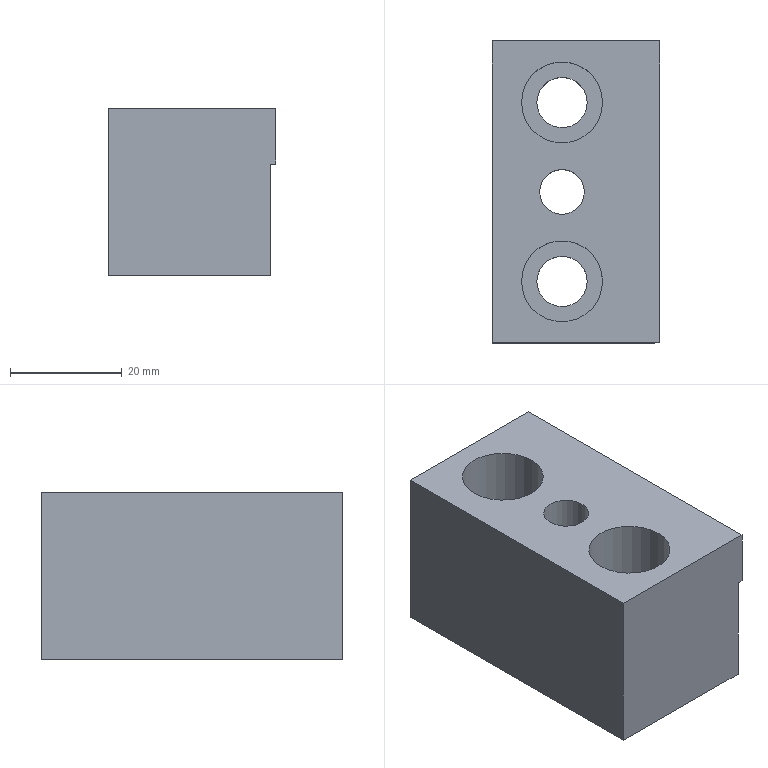Part | NX | features 23 2 | 1 solid | 15 faces | box 30 x 54 x 30 mm | volume 39961 mm3 | plane 10 | cylinder 5 | commonest cylinder face diameters 9 x2 14.5 x2 8.001 x1
STEP:
#1=CARTESIAN_POINT('',(3684.199,-436.,-14.5));
#2=VERTEX_POINT('',#1);
#3=CARTESIAN_POINT('',(3688.699,-436.,-14.5));
#4=DIRECTION('',(0.,0.,-1.));
#5=DIRECTION('',(-1.,0.,0.));
#6=AXIS2_PLACEMENT_3D('',#3,#4,#5);
#7=CIRCLE('',#6,4.5);
#8=EDGE_CURVE('',#2,#2,#7,.T.);
#9=ORIENTED_EDGE('',*,*,#8,.T.);
#10=EDGE_LOOP('',(#9));
#11=FACE_BOUND('',#10,.T.);
#12=CARTESIAN_POINT('',(3681.449,-436.,-14.5));
#13=VERTEX_POINT('',#12);
#14=CARTESIAN_POINT('',(3688.699,-436.,-14.5));
#15=DIRECTION('',(0.,0.,-1.));
#16=DIRECTION('',(-1.,0.,0.));
#17=AXIS2_PLACEMENT_3D('',#14,#15,#16);
#18=CIRCLE('',#17,7.25);
#19=EDGE_CURVE('',#13,#13,#18,.T.);
#20=ORIENTED_EDGE('',*,*,#19,.F.);
#21=EDGE_LOOP('',(#20));
#22=FACE_BOUND('',#21,.T.);
#23=CARTESIAN_POINT('',(3688.699,-436.,-14.5));
#24=DIRECTION('',(0.,0.,-1.));
#25=DIRECTION('',(-1.,0.,0.));
#26=AXIS2_PLACEMENT_3D('',#23,#24,#25);
#27=PLANE('',#26);
#28=ADVANCED_FACE('',(#11,#22),#27,.F.);
#29=CARTESIAN_POINT('',(3705.199,-393.,-13.5));
#30=VERTEX_POINT('',#29);
#31=CARTESIAN_POINT('',(3705.199,-447.,-13.5));
#32=VERTEX_POINT('',#31);
#33=CARTESIAN_POINT('',(3705.199,-407.5,-13.5));
#34=DIRECTION('',(0.,-1.,0.));
#35=VECTOR('',#34,1000.);
#36=LINE('',#33,#35);
#37=EDGE_CURVE('',#30,#32,#36,.T.);
#38=ORIENTED_EDGE('',*,*,#37,.F.);
#39=CARTESIAN_POINT('',(3706.199,-393.,-13.5));
#40=VERTEX_POINT('',#39);
#41=CARTESIAN_POINT('',(3678.699,-393.,-13.5));
#42=DIRECTION('',(-1.,0.,0.));
#43=VECTOR('',#42,1000.);
#44=LINE('',#41,#43);
#45=EDGE_CURVE('',#40,#30,#44,.T.);
#46=ORIENTED_EDGE('',*,*,#45,.F.);
#47=CARTESIAN_POINT('',(3706.199,-447.,-13.5));
#48=VERTEX_POINT('',#47);
#49=CARTESIAN_POINT('',(3706.199,-407.5,-13.5));
#50=DIRECTION('',(0.,1.,0.));
#51=VECTOR('',#50,1000.);
#52=LINE('',#49,#51);
#53=EDGE_CURVE('',#48,#40,#52,.T.);
#54=ORIENTED_EDGE('',*,*,#53,.F.);
#55=CARTESIAN_POINT('',(3706.199,-447.,-13.5));
#56=DIRECTION('',(1.,0.,0.));
#57=VECTOR('',#56,1000.);
#58=LINE('',#55,#57);
#59=EDGE_CURVE('',#32,#48,#58,.T.);
#60=ORIENTED_EDGE('',*,*,#59,.F.);
#61=EDGE_LOOP('',(#38,#46,#54,#60));
#62=FACE_BOUND('',#61,.T.);
#63=CARTESIAN_POINT('',(3691.199,-420.,-13.5));
#64=DIRECTION('',(0.,0.,1.));
#65=DIRECTION('',(1.,0.,0.));
#66=AXIS2_PLACEMENT_3D('',#63,#64,#65);
#67=PLANE('',#66);
#68=ADVANCED_FACE('',(#62),#67,.F.);
#69=ORIENTED_EDGE('',*,*,#8,.F.);
#70=EDGE_LOOP('',(#69));
#71=FACE_BOUND('',#70,.T.);
#72=CARTESIAN_POINT('',(3684.199,-436.,-33.5));
#73=VERTEX_POINT('',#72);
#74=CARTESIAN_POINT('',(3688.699,-436.,-33.5));
#75=DIRECTION('',(0.,0.,1.));
#76=DIRECTION('',(-1.,0.,0.));
#77=AXIS2_PLACEMENT_3D('',#74,#75,#76);
#78=CIRCLE('',#77,4.5);
#79=EDGE_CURVE('',#73,#73,#78,.T.);
#80=ORIENTED_EDGE('',*,*,#79,.F.);
#81=EDGE_LOOP('',(#80));
#82=FACE_BOUND('',#81,.T.);
#83=CARTESIAN_POINT('',(3688.699,-436.,-3.5));
#84=DIRECTION('',(0.,0.,-1.));
#85=DIRECTION('',(1.,0.,0.));
#86=AXIS2_PLACEMENT_3D('',#83,#84,#85);
#87=CYLINDRICAL_SURFACE('',#86,4.5);
#88=ADVANCED_FACE('',(#71,#82),#87,.F.);
#89=CARTESIAN_POINT('',(3705.199,-393.,-33.5));
#90=VERTEX_POINT('',#89);
#91=CARTESIAN_POINT('',(3705.199,-393.,-148.5));
#92=DIRECTION('',(0.,0.,1.));
#93=VECTOR('',#92,1000.);
#94=LINE('',#91,#93);
#95=EDGE_CURVE('',#90,#30,#94,.T.);
#96=ORIENTED_EDGE('',*,*,#95,.T.);
#97=ORIENTED_EDGE('',*,*,#37,.T.);
#98=CARTESIAN_POINT('',(3705.199,-447.,-33.5));
#99=VERTEX_POINT('',#98);
#100=CARTESIAN_POINT('',(3705.199,-447.,-25.5));
#101=DIRECTION('',(0.,0.,1.));
#102=VECTOR('',#101,1000.);
#103=LINE('',#100,#102);
#104=EDGE_CURVE('',#99,#32,#103,.T.);
#105=ORIENTED_EDGE('',*,*,#104,.F.);
#106=CARTESIAN_POINT('',(3705.199,-407.5,-33.5));
#107=DIRECTION('',(0.,-1.,0.));
#108=VECTOR('',#107,1000.);
#109=LINE('',#106,#108);
#110=EDGE_CURVE('',#90,#99,#109,.T.);
#111=ORIENTED_EDGE('',*,*,#110,.F.);
#112=EDGE_LOOP('',(#96,#97,#105,#111));
#113=FACE_BOUND('',#112,.T.);
#114=CARTESIAN_POINT('',(3705.199,-407.5,-148.5));
#115=DIRECTION('',(1.,0.,0.));
#116=DIRECTION('',(0.,0.,-1.));
#117=AXIS2_PLACEMENT_3D('',#114,#115,#116);
#118=PLANE('',#117);
#119=ADVANCED_FACE('',(#113),#118,.T.);
#120=ORIENTED_EDGE('',*,*,#19,.T.);
#121=EDGE_LOOP('',(#120));
#122=FACE_BOUND('',#121,.T.);
#123=CARTESIAN_POINT('',(3695.949,-436.,-3.5));
#124=VERTEX_POINT('',#123);
#125=CARTESIAN_POINT('',(3688.699,-436.,-3.5));
#126=DIRECTION('',(0.,0.,-1.));
#127=DIRECTION('',(1.,0.,0.));
#128=AXIS2_PLACEMENT_3D('',#125,#126,#127);
#129=CIRCLE('',#128,7.25);
#130=EDGE_CURVE('',#124,#124,#129,.T.);
#131=ORIENTED_EDGE('',*,*,#130,.F.);
#132=EDGE_LOOP('',(#131));
#133=FACE_BOUND('',#132,.T.);
#134=CARTESIAN_POINT('',(3688.699,-436.,-3.5));
#135=DIRECTION('',(0.,0.,-1.));
#136=DIRECTION('',(1.,0.,0.));
#137=AXIS2_PLACEMENT_3D('',#134,#135,#136);
#138=CYLINDRICAL_SURFACE('',#137,7.25);
#139=ADVANCED_FACE('',(#122,#133),#138,.F.);
#140=CARTESIAN_POINT('',(3684.699,-420.,-33.5));
#141=VERTEX_POINT('',#140);
#142=CARTESIAN_POINT('',(3688.699,-420.,-33.5));
#143=DIRECTION('',(0.,0.,-1.));
#144=DIRECTION('',(-1.,0.,0.));
#145=AXIS2_PLACEMENT_3D('',#142,#143,#144);
#146=CIRCLE('',#145,4.);
#147=EDGE_CURVE('',#141,#141,#146,.T.);
#148=ORIENTED_EDGE('',*,*,#147,.T.);
#149=EDGE_LOOP('',(#148));
#150=FACE_BOUND('',#149,.T.);
#151=CARTESIAN_POINT('',(3692.7,-420.,-3.5));
#152=VERTEX_POINT('',#151);
#153=CARTESIAN_POINT('',(3688.699,-420.,-3.5));
#154=DIRECTION('',(0.,0.,1.));
#155=DIRECTION('',(1.,0.,0.));
#156=AXIS2_PLACEMENT_3D('',#153,#154,#155);
#157=CIRCLE('',#156,4.);
#158=EDGE_CURVE('',#152,#152,#157,.T.);
#159=ORIENTED_EDGE('',*,*,#158,.T.);
#160=EDGE_LOOP('',(#159));
#161=FACE_BOUND('',#160,.T.);
#162=CARTESIAN_POINT('',(3688.699,-420.,51.5));
#163=DIRECTION('',(0.,0.,-1.));
#164=DIRECTION('',(-1.,0.,0.));
#165=AXIS2_PLACEMENT_3D('',#162,#163,#164);
#166=CYLINDRICAL_SURFACE('',#165,4.);
#167=ADVANCED_FACE('',(#150,#161),#166,.F.);
#168=CARTESIAN_POINT('',(3676.199,-447.,-3.5));
#169=VERTEX_POINT('',#168);
#170=CARTESIAN_POINT('',(3676.199,-393.,-3.5));
#171=VERTEX_POINT('',#170);
#172=CARTESIAN_POINT('',(3676.199,-383.325,-3.5));
#173=DIRECTION('',(0.,1.,0.));
#174=VECTOR('',#173,1000.);
#175=LINE('',#172,#174);
#176=EDGE_CURVE('',#169,#171,#175,.T.);
#177=ORIENTED_EDGE('',*,*,#176,.T.);
#178=CARTESIAN_POINT('',(3676.199,-393.,-33.5));
#179=VERTEX_POINT('',#178);
#180=CARTESIAN_POINT('',(3676.199,-393.,-148.5));
#181=DIRECTION('',(0.,0.,-1.));
#182=VECTOR('',#181,1000.);
#183=LINE('',#180,#182);
#184=EDGE_CURVE('',#171,#179,#183,.T.);
#185=ORIENTED_EDGE('',*,*,#184,.T.);
#186=CARTESIAN_POINT('',(3676.199,-447.,-33.5));
#187=VERTEX_POINT('',#186);
#188=CARTESIAN_POINT('',(3676.199,-407.5,-33.5));
#189=DIRECTION('',(0.,-1.,0.));
#190=VECTOR('',#189,1000.);
#191=LINE('',#188,#190);
#192=EDGE_CURVE('',#179,#187,#191,.T.);
#193=ORIENTED_EDGE('',*,*,#192,.T.);
#194=CARTESIAN_POINT('',(3676.199,-447.,-25.5));
#195=DIRECTION('',(0.,0.,1.));
#196=VECTOR('',#195,1000.);
#197=LINE('',#194,#196);
#198=EDGE_CURVE('',#187,#169,#197,.T.);
#199=ORIENTED_EDGE('',*,*,#198,.T.);
#200=EDGE_LOOP('',(#177,#185,#193,#199));
#201=FACE_BOUND('',#200,.T.);
#202=CARTESIAN_POINT('',(3676.199,-407.5,-25.5));
#203=DIRECTION('',(-1.,0.,0.));
#204=DIRECTION('',(0.,0.,1.));
#205=AXIS2_PLACEMENT_3D('',#202,#203,#204);
#206=PLANE('',#205);
#207=ADVANCED_FACE('',(#201),#206,.T.);
#208=ORIENTED_EDGE('',*,*,#104,.T.);
#209=ORIENTED_EDGE('',*,*,#59,.T.);
#210=CARTESIAN_POINT('',(3706.199,-447.,-3.5));
#211=VERTEX_POINT('',#210);
#212=CARTESIAN_POINT('',(3706.199,-447.,-148.5));
#213=DIRECTION('',(0.,0.,1.));
#214=VECTOR('',#213,1000.);
#215=LINE('',#212,#214);
#216=EDGE_CURVE('',#48,#211,#215,.T.);
#217=ORIENTED_EDGE('',*,*,#216,.T.);
#218=CARTESIAN_POINT('',(2177.271,-447.,-3.5));
#219=DIRECTION('',(1.,0.,0.));
#220=VECTOR('',#219,1000.);
#221=LINE('',#218,#220);
#222=EDGE_CURVE('',#169,#211,#221,.T.);
#223=ORIENTED_EDGE('',*,*,#222,.F.);
#224=ORIENTED_EDGE('',*,*,#198,.F.);
#225=CARTESIAN_POINT('',(3706.199,-447.,-33.5));
#226=DIRECTION('',(1.,0.,0.));
#227=VECTOR('',#226,1000.);
#228=LINE('',#225,#227);
#229=EDGE_CURVE('',#187,#99,#228,.T.);
#230=ORIENTED_EDGE('',*,*,#229,.T.);
#231=EDGE_LOOP('',(#208,#209,#217,#223,#224,#230));
#232=FACE_BOUND('',#231,.T.);
#233=CARTESIAN_POINT('',(3706.199,-447.,-25.5));
#234=DIRECTION('',(0.,-1.,0.));
#235=DIRECTION('',(0.,0.,-1.));
#236=AXIS2_PLACEMENT_3D('',#233,#234,#235);
#237=PLANE('',#236);
#238=ADVANCED_FACE('',(#232),#237,.T.);
#239=ORIENTED_EDGE('',*,*,#53,.T.);
#240=CARTESIAN_POINT('',(3706.199,-393.,-3.5));
#241=VERTEX_POINT('',#240);
#242=CARTESIAN_POINT('',(3706.199,-393.,-148.5));
#243=DIRECTION('',(0.,0.,1.));
#244=VECTOR('',#243,1000.);
#245=LINE('',#242,#244);
#246=EDGE_CURVE('',#40,#241,#245,.T.);
#247=ORIENTED_EDGE('',*,*,#246,.T.);
#248=CARTESIAN_POINT('',(3706.199,-407.5,-3.5));
#249=DIRECTION('',(0.,-1.,0.));
#250=VECTOR('',#249,1000.);
#251=LINE('',#248,#250);
#252=EDGE_CURVE('',#241,#211,#251,.T.);
#253=ORIENTED_EDGE('',*,*,#252,.T.);
#254=ORIENTED_EDGE('',*,*,#216,.F.);
#255=EDGE_LOOP('',(#239,#247,#253,#254));
#256=FACE_BOUND('',#255,.T.);
#257=CARTESIAN_POINT('',(3706.199,-407.5,-148.5));
#258=DIRECTION('',(1.,0.,0.));
#259=DIRECTION('',(0.,0.,-1.));
#260=AXIS2_PLACEMENT_3D('',#257,#258,#259);
#261=PLANE('',#260);
#262=ADVANCED_FACE('',(#256),#261,.T.);
#263=ORIENTED_EDGE('',*,*,#184,.F.);
#264=CARTESIAN_POINT('',(3678.699,-393.,-3.5));
#265=DIRECTION('',(1.,0.,0.));
#266=VECTOR('',#265,1000.);
#267=LINE('',#264,#266);
#268=EDGE_CURVE('',#171,#241,#267,.T.);
#269=ORIENTED_EDGE('',*,*,#268,.T.);
#270=ORIENTED_EDGE('',*,*,#246,.F.);
#271=ORIENTED_EDGE('',*,*,#45,.T.);
#272=ORIENTED_EDGE('',*,*,#95,.F.);
#273=CARTESIAN_POINT('',(3706.199,-393.,-33.5));
#274=DIRECTION('',(1.,0.,0.));
#275=VECTOR('',#274,1000.);
#276=LINE('',#273,#275);
#277=EDGE_CURVE('',#179,#90,#276,.T.);
#278=ORIENTED_EDGE('',*,*,#277,.F.);
#279=EDGE_LOOP('',(#263,#269,#270,#271,#272,#278));
#280=FACE_BOUND('',#279,.T.);
#281=CARTESIAN_POINT('',(3678.699,-393.,-148.5));
#282=DIRECTION('',(0.,1.,0.));
#283=DIRECTION('',(0.,0.,1.));
#284=AXIS2_PLACEMENT_3D('',#281,#282,#283);
#285=PLANE('',#284);
#286=ADVANCED_FACE('',(#280),#285,.T.);
#287=CARTESIAN_POINT('',(3695.949,-404.,-3.5));
#288=VERTEX_POINT('',#287);
#289=CARTESIAN_POINT('',(3688.699,-404.,-3.5));
#290=DIRECTION('',(0.,0.,-1.));
#291=DIRECTION('',(1.,0.,0.));
#292=AXIS2_PLACEMENT_3D('',#289,#290,#291);
#293=CIRCLE('',#292,7.25);
#294=EDGE_CURVE('',#288,#288,#293,.T.);
#295=ORIENTED_EDGE('',*,*,#294,.T.);
#296=EDGE_LOOP('',(#295));
#297=FACE_BOUND('',#296,.T.);
#298=ORIENTED_EDGE('',*,*,#268,.F.);
#299=ORIENTED_EDGE('',*,*,#176,.F.);
#300=ORIENTED_EDGE('',*,*,#222,.T.);
#301=ORIENTED_EDGE('',*,*,#252,.F.);
#302=EDGE_LOOP('',(#298,#299,#300,#301));
#303=FACE_BOUND('',#302,.T.);
#304=ORIENTED_EDGE('',*,*,#158,.F.);
#305=EDGE_LOOP('',(#304));
#306=FACE_BOUND('',#305,.T.);
#307=ORIENTED_EDGE('',*,*,#130,.T.);
#308=EDGE_LOOP('',(#307));
#309=FACE_BOUND('',#308,.T.);
#310=CARTESIAN_POINT('',(2177.271,-383.325,-3.5));
#311=DIRECTION('',(0.,0.,1.));
#312=DIRECTION('',(1.,0.,0.));
#313=AXIS2_PLACEMENT_3D('',#310,#311,#312);
#314=PLANE('',#313);
#315=ADVANCED_FACE('',(#297,#303,#306,#309),#314,.T.);
#316=CARTESIAN_POINT('',(3684.199,-404.,-33.5));
#317=VERTEX_POINT('',#316);
#318=CARTESIAN_POINT('',(3688.699,-404.,-33.5));
#319=DIRECTION('',(0.,0.,1.));
#320=DIRECTION('',(-1.,0.,0.));
#321=AXIS2_PLACEMENT_3D('',#318,#319,#320);
#322=CIRCLE('',#321,4.5);
#323=EDGE_CURVE('',#317,#317,#322,.T.);
#324=ORIENTED_EDGE('',*,*,#323,.T.);
#325=EDGE_LOOP('',(#324));
#326=FACE_BOUND('',#325,.T.);
#327=ORIENTED_EDGE('',*,*,#147,.F.);
#328=EDGE_LOOP('',(#327));
#329=FACE_BOUND('',#328,.T.);
#330=ORIENTED_EDGE('',*,*,#277,.T.);
#331=ORIENTED_EDGE('',*,*,#110,.T.);
#332=ORIENTED_EDGE('',*,*,#229,.F.);
#333=ORIENTED_EDGE('',*,*,#192,.F.);
#334=EDGE_LOOP('',(#330,#331,#332,#333));
#335=FACE_BOUND('',#334,.T.);
#336=ORIENTED_EDGE('',*,*,#79,.T.);
#337=EDGE_LOOP('',(#336));
#338=FACE_BOUND('',#337,.T.);
#339=CARTESIAN_POINT('',(3706.199,-407.5,-33.5));
#340=DIRECTION('',(0.,0.,-1.));
#341=DIRECTION('',(-1.,0.,0.));
#342=AXIS2_PLACEMENT_3D('',#339,#340,#341);
#343=PLANE('',#342);
#344=ADVANCED_FACE('',(#326,#329,#335,#338),#343,.T.);
#345=CARTESIAN_POINT('',(3684.199,-404.,-14.5));
#346=VERTEX_POINT('',#345);
#347=CARTESIAN_POINT('',(3688.699,-404.,-14.5));
#348=DIRECTION('',(0.,0.,-1.));
#349=DIRECTION('',(-1.,0.,0.));
#350=AXIS2_PLACEMENT_3D('',#347,#348,#349);
#351=CIRCLE('',#350,4.5);
#352=EDGE_CURVE('',#346,#346,#351,.T.);
#353=ORIENTED_EDGE('',*,*,#352,.T.);
#354=EDGE_LOOP('',(#353));
#355=FACE_BOUND('',#354,.T.);
#356=CARTESIAN_POINT('',(3681.449,-404.,-14.5));
#357=VERTEX_POINT('',#356);
#358=CARTESIAN_POINT('',(3688.699,-404.,-14.5));
#359=DIRECTION('',(0.,0.,-1.));
#360=DIRECTION('',(-1.,0.,0.));
#361=AXIS2_PLACEMENT_3D('',#358,#359,#360);
#362=CIRCLE('',#361,7.25);
#363=EDGE_CURVE('',#357,#357,#362,.T.);
#364=ORIENTED_EDGE('',*,*,#363,.F.);
#365=EDGE_LOOP('',(#364));
#366=FACE_BOUND('',#365,.T.);
#367=CARTESIAN_POINT('',(3688.699,-404.,-14.5));
#368=DIRECTION('',(0.,0.,-1.));
#369=DIRECTION('',(-1.,0.,0.));
#370=AXIS2_PLACEMENT_3D('',#367,#368,#369);
#371=PLANE('',#370);
#372=ADVANCED_FACE('',(#355,#366),#371,.F.);
#373=ORIENTED_EDGE('',*,*,#363,.T.);
#374=EDGE_LOOP('',(#373));
#375=FACE_BOUND('',#374,.T.);
#376=ORIENTED_EDGE('',*,*,#294,.F.);
#377=EDGE_LOOP('',(#376));
#378=FACE_BOUND('',#377,.T.);
#379=CARTESIAN_POINT('',(3688.699,-404.,-3.5));
#380=DIRECTION('',(0.,0.,-1.));
#381=DIRECTION('',(1.,0.,0.));
#382=AXIS2_PLACEMENT_3D('',#379,#380,#381);
#383=CYLINDRICAL_SURFACE('',#382,7.25);
#384=ADVANCED_FACE('',(#375,#378),#383,.F.);
#385=ORIENTED_EDGE('',*,*,#352,.F.);
#386=EDGE_LOOP('',(#385));
#387=FACE_BOUND('',#386,.T.);
#388=ORIENTED_EDGE('',*,*,#323,.F.);
#389=EDGE_LOOP('',(#388));
#390=FACE_BOUND('',#389,.T.);
#391=CARTESIAN_POINT('',(3688.699,-404.,-3.5));
#392=DIRECTION('',(0.,0.,-1.));
#393=DIRECTION('',(1.,0.,0.));
#394=AXIS2_PLACEMENT_3D('',#391,#392,#393);
#395=CYLINDRICAL_SURFACE('',#394,4.5);
#396=ADVANCED_FACE('',(#387,#390),#395,.F.);
#397=CLOSED_SHELL('',(#28,#68,#88,#119,#139,#167,#207,#238,#262,#286,#315,#344,#372,#384,#396));
#398=MANIFOLD_SOLID_BREP('',#397);
#399=(LENGTH_UNIT()NAMED_UNIT(*)SI_UNIT(.MILLI.,.METRE.));
#400=UNCERTAINTY_MEASURE_WITH_UNIT(LENGTH_MEASURE(0.00001),#399,'','');
#401=(NAMED_UNIT(*)PLANE_ANGLE_UNIT()SI_UNIT($,.RADIAN.));
#402=(NAMED_UNIT(*)SI_UNIT($,.STERADIAN.)SOLID_ANGLE_UNIT());
#403=(GEOMETRIC_REPRESENTATION_CONTEXT(3)GLOBAL_UNCERTAINTY_ASSIGNED_CONTEXT((#400))GLOBAL_UNIT_ASSIGNED_CONTEXT((#399,#401,#402))REPRESENTATION_CONTEXT('',''));
#404=ADVANCED_BREP_SHAPE_REPRESENTATION('',(#398),#403);